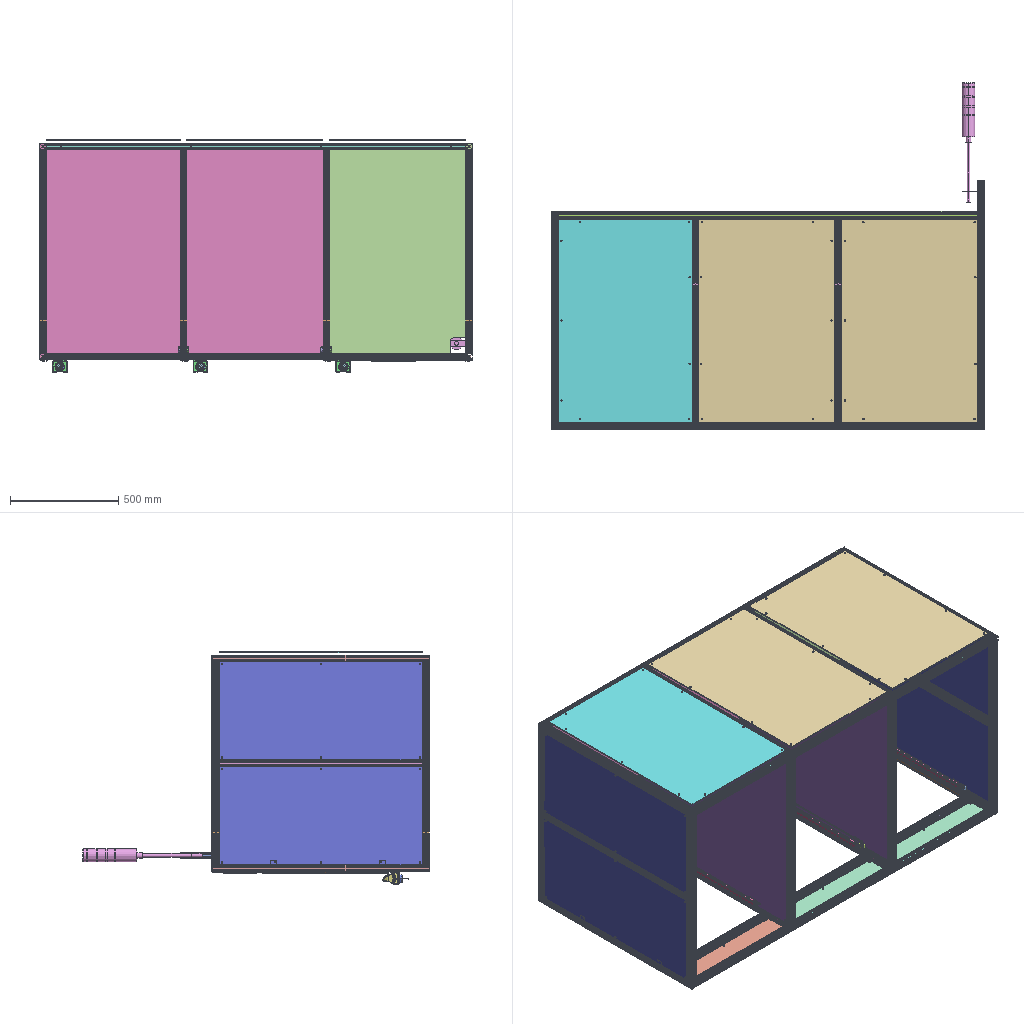Assembly | SolidWorks | 37 different items | 93 placed | box 2000 x 1600 x 1073 mm
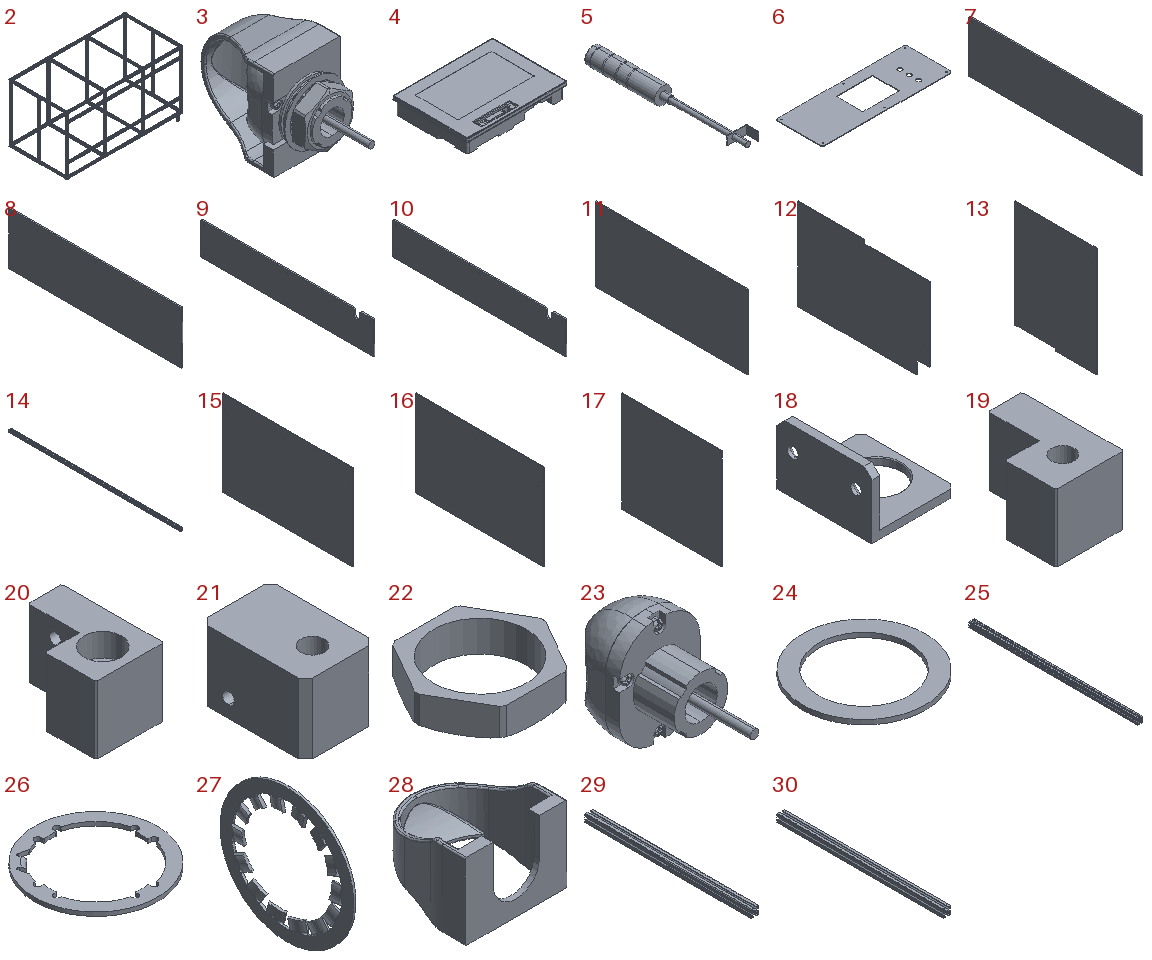Parts list (item | name | quantity | parent item | size | volume | features):
1 | (subassembly) | x2 | - | - | - | features RefAxis 3
2 | (subassembly) | x1 | - | 2000 x 1000 x 1150 mm | 9577291 mm3 | -
3 | (subassembly) | x3 | - | 51 x 119.5 x 68 mm | 99680 mm3 | features RefAxis 3
4 | - | x1 | - | 203 x 152 x 35.35 mm | 852828 mm3 | features BaseBody 1
5 | - | x1 | - | 74 x 551.1 x 60 mm | 791689 mm3 | features Boss 11, ICE 3, BossThin 1, Cut 1, Fillet 1, Shell 1, Sweep 1
6 | - | x1 | - | 690 x 250 x 3 mm | 429850 mm3 | features ICE 2, Extrusion 1, Fillet 1, HoleWzd 1
7 | - | x1 | - | 5 x 628 x 188 mm | 589462 mm3 | features Chamfer 1, Extrusion 1, ICE 1
8 | - | x1 | - | 5 x 618 x 188 mm | 580062 mm3 | features Chamfer 1, Extrusion 1, ICE 1
9 | - | x2 | - | 5 x 628 x 118 mm | 366831 mm3 | features Chamfer 2, ICE 2, Extrusion 1
10 | - | x1 | - | 5 x 628 x 118 mm | 366831 mm3 | features Chamfer 2, ICE 2, Extrusion 1
11 | - | x4 | - | 5 x 937 x 453 mm | 2121447 mm3 | features Chamfer 1, Extrusion 1, ICE 1
12 | - | x1 | - | 5 x 1000 x 690 mm | 3324176 mm3 | features Chamfer 2, Fillet 2, ICE 2, Cut 1, Extrusion 1, HoleWzd 1
13 | - | x1 | - | 5 x 1000 x 1340 mm | 6624000 mm3 | features Chamfer 2, Fillet 2, ICE 2, Extrusion 1
14 | - | x2 | in 2 | 30 x 1940 x 30 mm | 645123 mm3 | features Extrusion 1
15 | - | x1 | - | 5 x 938 x 618 mm | 2897138 mm3 | features Chamfer 1, Extrusion 1, ICE 1
16 | - | x2 | - | 5 x 938 x 628 mm | 2944038 mm3 | features Chamfer 1, Extrusion 1, ICE 1
17 | - | x2 | - | 5 x 937 x 938 mm | 4393672 mm3 | features Chamfer 1, Extrusion 1, ICE 1
18 | - | x3 | - | 53 x 60 x 40 mm | 21818 mm3 | features Chamfer 3, Extrusion 1, HoleWzd 1, ICE 1
19 | - | x2 | - | 20 x 30 x 20 mm | 7804 mm3 | features HoleWzd 2, Chamfer 1, Extrusion 1, ICE 1
20 | - | x2 | - | 20 x 30 x 20 mm | 7804 mm3 | features MirrorStock 1
21 | - | x4 | - | 20 x 30 x 20 mm | 10571 mm3 | features HoleWzd 2, Chamfer 1, Extrusion 1
22 | - | x3 | in 3 | 40.6 x 36 x 10 mm | 4057 mm3 | features RefAxis 3, BaseBody 1
23 | - | x3 | in 3 | 45 x 85.792 x 60 mm | 63985 mm3 | features RefAxis 3, BaseBody 1
24 | - | x3 | in 3 | 42 x 42 x 1.6 mm | 1009 mm3 | features RefAxis 3, BaseBody 1
25 | - | x6 | in 2 | 30 x 940 x 30 mm | 312585 mm3 | features Extrusion 1
26 | - | x3 | in 3 | 38 x 38 x 3.2 mm | 486.379 mm3 | features RefAxis 3, BaseBody 1
27 | - | x3 | in 3 | 2 x 46 x 46 mm | 665.952 mm3 | features RefAxis 3, BaseBody 1
28 | - | x3 | in 3 | 68 x 70 x 51 mm | 29414 mm3 | features RefAxis 3, BaseBody 1
29 | - | x2 | in 2 | 30 x 620 x 30 mm | 206173 mm3 | features Extrusion 1
30 | - | x2 | in 2 | 30 x 630 x 30 mm | 209499 mm3 | features Extrusion 1
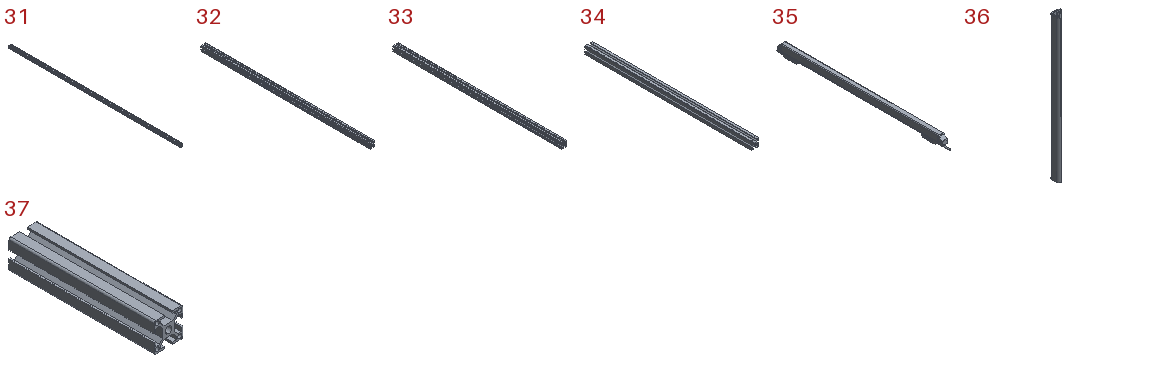31 | - | x2 | in 2 | 30 x 1940 x 30 mm | 644146 mm3 | features Extrusion 1, HoleWzd 1
32 | - | x4 | in 2 | 30 x 1000 x 30 mm | 332538 mm3 | features Extrusion 1
33 | - | x8 | in 2 | 30 x 940 x 30 mm | 311608 mm3 | features Extrusion 1, HoleWzd 1
34 | - | x2 | in 2 | 30 x 630 x 30 mm | 209499 mm3 | features Extrusion 1
35 | - | x6 | - | 15 x 516.175 x 30 mm | 163746 mm3 | features BaseBody 3
36 | - | x4 | - | 37 x 37 x 530 mm | 171468 mm3 | features BaseBody 1, MoveFace 1
37 | - | x1 | in 2 | 30 x 150 x 30 mm | 49881 mm3 | features Extrusion 1
Mates (type | each side: item.copy, entity, surface, feature):
In the top assembly
Coincident | 32.1 face plane Extrude 1 | 6.1 face plane Boss-Extrude 1
Coincident | 14.1 face plane Extrude 1 | 6.1 face plane Boss-Extrude 1
Coincident | 6.1 face plane Boss-Extrude 1 | 4.1 face plane Import 1
Coincident | 6.1 face plane Cut-Extrude 1 | 4.1 face plane Import 1 | 2 times
Coincident | 37.1 face plane Extrude 1 | 5.1 face plane Extrude-Thin Wall 1
Width | 37.1 face plane Extrude 1 | 37.1 face plane Extrude 1 | 5.1 face plane Extrude-Thin Wall 1 | 5.1 face plane Extrude-Thin Wall 1
DistanceDim | 5.1 face plane Extrude 11 | 33.1 face plane Extrude 1
Coincident | 31.1 face plane Extrude 1 | 9.1 face plane Boss-Extrude 1
DistanceDim | 32.1 face plane Extrude 1 | 9.1 face plane Boss-Extrude 1
Coincident | 33.2 face plane Extrude 1 | 11.1 face plane Boss-Extrude 1
DistanceDim | 33.2 face plane Extrude 1 | 11.1 face plane Boss-Extrude 1
DistanceDim | 11.1 face plane Boss-Extrude 1 | 25.1 face plane Extrude 1
Coincident | assembly face | 12.1 face plane Boss-Extrude 1
Coincident | 32.2 face plane Extrude 1 | 12.1 face plane Boss-Extrude 1
Coincident | 33.1 face plane Extrude 1 | 12.1 face plane Boss-Extrude 1
Coincident | 33.3 face plane Extrude 1 | 12.1 face plane Boss-Extrude 1
Coincident | 33.4 face plane Extrude 1 | 13.1 face plane Boss-Extrude 1
Coincident | 14.2 face plane Extrude 1 | 13.1 face plane Boss-Extrude 1
Concentric | 19.1 face cylinder M4 Tapped Hole 1 | 35.1 face cylinder Input 2
Coincident | 19.1 face plane Cut-Extrude 1 | 35.1 face plane Input 2
Concentric | 20.1 face cylinder XXXXXXXXXXXXXXVJTL6_Mirror | 35.1 edge
Coincident | 20.1 face plane XXXXXXXXXXXXXXVJTL6_Mirror | 35.1 face plane Input 1
Parallel | 19.1 face plane Boss-Extrude 1 | 35.1 face plane Input 3
Parallel | 20.1 face plane XXXXXXXXXXXXXXVJTL6_Mirror | 35.1 face plane Input 3
Coincident | 19.2 face plane Cut-Extrude 1 | 35.2 face plane Input 2
Concentric | 20.2 face cylinder XXXXXXXXXXXXXXVJTL6_Mirror | 35.2 edge
Concentric | 19.2 face cylinder M4 Tapped Hole 1 | 35.2 face cylinder Input 2
Parallel | 19.2 face plane Boss-Extrude 1 | 35.2 face plane Input 3
Parallel | 20.2 face plane XXXXXXXXXXXXXXVJTL6_Mirror | 35.2 face plane Input 3
Coincident | 20.2 face plane XXXXXXXXXXXXXXVJTL6_Mirror | 35.2 face plane Input 1
Coincident | 32.1 face plane Extrude 1 | 19.1 face plane Boss-Extrude 1
Coincident | 32.1 face plane Extrude 1 | 35.1 face plane Input 3
Coincident | 25.2 face plane Extrude 1 | 36.1 face plane Input 1 | 2 times
Coincident | 32.1 face plane Extrude 1 | 36.2 face plane Input 1 | 2 times
Coincident | 36.1 face plane Input 1 | 36.2 face plane Input 1
Coincident | 25.3 face plane Extrude 1 | 36.3 face plane Input 1 | 2 times
Coincident | 32.3 face plane Extrude 1 | 36.4 face plane Input 1 | 2 times
DistanceDim | 32.3 face plane Extrude 1 | 20.2 face plane XXXXXXXXXXXXXXVJTL6_Mirror
Coincident | 32.3 face plane Extrude 1 | 20.2 face plane XXXXXXXXXXXXXXVJTL6_Mirror
DistanceDim | 9.1 face plane Boss-Extrude 1 | 31.1 face plane Extrude 1
Concentric | 35.3 face cylinder Input 2 | 21.1 face cylinder M4 Tapped Hole 1
Coincident | 35.3 face plane Input 2 | 21.1 face plane Boss-Extrude 1
Concentric | 35.4 face cylinder Input 1 | 21.1 face cylinder M4 Tapped Hole 1
Coincident | 35.4 face plane Input 1 | 21.1 face plane Boss-Extrude 1
Parallel | 35.3 face plane Input 3 | 21.1 face plane Boss-Extrude 1
Coincident | 35.3 face plane Input 3 | 35.4 face plane Input 3
Concentric | 35.4 face cylinder Input 2 | 21.2 face cylinder M4 Tapped Hole 1
Coincident | 35.4 face plane Input 2 | 21.2 face plane Boss-Extrude 1
Coincident | 21.3 face plane Boss-Extrude 1 | 35.5 face plane Input 1
Concentric | 21.3 face cylinder M4 Tapped Hole 1 | 35.5 face cylinder Input 1
Coincident | 21.3 face plane Boss-Extrude 1 | 35.6 face plane Input 2
Parallel | 21.3 face plane Boss-Extrude 1 | 35.6 face plane Input 3
Concentric | 21.3 face cylinder M4 Tapped Hole 1 | 35.6 face cylinder Input 2
Coincident | 35.5 face plane Input 3 | 35.6 face plane Input 3
Concentric | 21.4 face cylinder M4 Tapped Hole 1 | 35.5 face cylinder Input 2
Coincident | 21.4 face plane Boss-Extrude 1 | 35.5 face plane Input 2
Coincident | 25.2 face plane Extrude 1 | 21.1 face plane Boss-Extrude 1
DistanceDim | 21.1 face plane Boss-Extrude 1 | 25.2 face plane Extrude 1
Coincident | 25.3 face plane Extrude 1 | 21.3 face plane Boss-Extrude 1
DistanceDim | 21.3 face plane Boss-Extrude 1 | 25.3 face plane Extrude 1
Coincident | 19.1 face plane Boss-Extrude 1 | 21.1 face plane Boss-Extrude 1
Coincident | 21.1 face plane Boss-Extrude 1 | 21.3 face plane Boss-Extrude 1
Coincident | 20.2 face plane XXXXXXXXXXXXXXVJTL6_Mirror | 21.3 face plane Boss-Extrude 1
Coincident | 36.1 face plane Input 1 | 21.1 face plane Boss-Extrude 1
Coincident | 6.1 face plane Boss-Extrude 1 | 32.1 face plane Extrude 1
Coincident | 11.2 face plane Boss-Extrude 1 | 11.1 face plane Boss-Extrude 1
DistanceDim | 11.2 face plane Boss-Extrude 1 | 33.1 face plane Extrude 1
DistanceDim | 11.2 face plane Boss-Extrude 1 | 32.2 face plane Extrude 1
Coincident | 32.3 face plane Extrude 1 | 11.3 face plane Boss-Extrude 1
DistanceDim | 11.3 face plane Boss-Extrude 1 | 33.4 face plane Extrude 1
DistanceDim | 11.3 face plane Boss-Extrude 1 | 32.3 face plane Extrude 1
Coincident | 11.3 face plane Boss-Extrude 1 | 11.4 face plane Boss-Extrude 1
DistanceDim | 33.4 face plane Extrude 1 | 11.4 face plane Boss-Extrude 1
DistanceDim | 11.4 face plane Boss-Extrude 1 | 32.4 face plane Extrude 1
Coincident | 25.4 face plane Extrude 1 | 17.1 face plane Boss-Extrude 1
DistanceDim | 33.3 face plane Extrude 1 | 17.1 face plane Boss-Extrude 1
DistanceDim | 25.4 face plane Extrude 1 | 17.1 face plane Boss-Extrude 1
Coincident | 25.5 face plane Extrude 1 | 17.2 face plane Boss-Extrude 1
DistanceDim | 17.2 face plane Boss-Extrude 1 | 33.5 face plane Extrude 1
DistanceDim | 25.3 face plane Extrude 1 | 17.2 face plane Boss-Extrude 1
Coincident | 9.1 face plane Boss-Extrude 1 | 9.2 face plane Boss-Extrude 1
DistanceDim | 9.2 face plane Boss-Extrude 1 | 30.1 face plane Extrude 1
DistanceDim | 9.2 face plane Boss-Extrude 1 | 25.3 face plane Extrude 1
Coincident | 9.2 face plane Boss-Extrude 1 | 10.1 face plane Boss-Extrude 1
DistanceDim | 10.1 face plane Boss-Extrude 1 | 29.1 face plane Extrude 1
DistanceDim | 10.1 face plane Boss-Extrude 1 | 32.3 face plane Extrude 1
Concentric | 18.1 face cylinder Cut-Extrude 1 | 24.1 face cylinder Input 1
Coincident | 18.1 face plane Boss-Extrude 1 | 28.1 face plane Input 1
Parallel | 18.1 face plane Boss-Extrude 1 | 28.1 face plane Input 1
Coincident | 34.1 face plane Extrude 1 | 18.1 face plane Boss-Extrude 1 | 2 times
DistanceDim | 23.1 face cylinder Input 1 | 25.2 face plane Extrude 1
Concentric | 18.2 face cylinder Cut-Extrude 1 | 26.1 face cylinder Input 1
Coincident | 18.2 face plane Boss-Extrude 1 | 28.2 face plane Input 1
Parallel | 18.2 face plane Boss-Extrude 1 | 28.2 face plane Input 1
Concentric | 18.3 face cylinder Cut-Extrude 1 | 26.2 face cylinder Input 1
Coincident | 18.3 face plane Boss-Extrude 1 | 28.3 face plane Input 1
Parallel | 18.3 face plane Boss-Extrude 1 | 28.3 face plane Input 1
Coincident | 30.1 face plane Extrude 1 | 18.2 face plane Boss-Extrude 1 | 2 times
DistanceDim | 23.2 face cylinder Input 1 | 25.3 face plane Extrude 1
Coincident | 29.1 face plane Extrude 1 | 18.3 face plane Boss-Extrude 1 | 2 times
DistanceDim | 23.3 face cylinder Input 1 | 32.3 face plane Extrude 1
DistanceDim | 16.1 face plane Boss-Extrude 1 | 14.2 face plane Extrude 1
DistanceDim | 16.1 face plane Boss-Extrude 1 | 25.5 face plane Extrude 1
Coincident | 16.1 face plane Boss-Extrude 1 | 16.2 face plane Boss-Extrude 1
DistanceDim | 16.2 face plane Boss-Extrude 1 | 14.2 face plane Extrude 1
DistanceDim | 16.2 face plane Boss-Extrude 1 | 32.2 face plane Extrude 1
Coincident | 14.1 face plane Extrude 1 | 7.1 face plane Boss-Extrude 1
DistanceDim | 7.1 face plane Boss-Extrude 1 | 30.2 face plane Extrude 1
DistanceDim | 7.1 face plane Boss-Extrude 1 | 25.3 face plane Extrude 1
Coincident | 7.1 face plane Boss-Extrude 1 | 8.1 face plane Boss-Extrude 1
DistanceDim | 8.1 face plane Boss-Extrude 1 | 14.1 face plane Extrude 1
DistanceDim | 8.1 face plane Boss-Extrude 1 | 32.3 face plane Extrude 1
Coincident | assembly face | 4.1 face plane Import 1 | 3 times
Coincident | 16.1 face plane Boss-Extrude 1 | 15.1 face plane Boss-Extrude 1
DistanceDim | 15.1 face plane Boss-Extrude 1 | 14.2 face plane Extrude 1
DistanceDim | 15.1 face plane Boss-Extrude 1 | 32.4 face plane Extrude 1
In subassembly 2
Coincident | 31.2 face plane Extrude 1 | 25.6 face plane Extrude 1 | 2 times
Coincident | 32.5 face plane Extrude 1 | 33.6 face plane Extrude 1 | 3 times
Coincident | 14.3 face plane Extrude 1 | 32.6 face plane Extrude 1 | 3 times
DistanceDim | 31.3 face plane Extrude 1 | 14.3 face plane Extrude 1
Coincident | 14.4 face plane Extrude 1 | 32.5 face plane Extrude 1 | 3 times
Coincident | 31.2 face plane Extrude 1 | 25.7 face plane Extrude 1 | 2 times
Coincident | 14.4 face plane Extrude 1 | 33.7 face plane Extrude 1 | 2 times
Coincident | 31.2 face plane Extrude 1 | 32.5 face plane Extrude 1
Coincident | 31.2 face plane Extrude 1 | 31.3 face plane Extrude 1
Coincident | 32.6 face plane Extrude 1 | 33.8 face plane Extrude 1 | 3 times
Coincident | 33.8 face plane Extrude 1 | 25.8 face plane Extrude 1 | 2 times
Width | 32.5 face plane Extrude 1 | 32.6 face plane Extrude 1 | 25.8 face plane Extrude 1 | 25.8 face plane Extrude 1
Coincident | 32.6 face plane Extrude 1 | 34.2 face plane Extrude 1 | 2 times
Coincident | 31.3 face plane Extrude 1 | 25.9 face plane Extrude 1 | 2 times
Coincident | 14.4 face plane Extrude 1 | 33.9 face plane Extrude 1 | 2 times
Coincident | 31.3 face plane Extrude 1 | 32.7 face plane Extrude 1 | 3 times
Coincident | 31.2 face plane Extrude 1 | 32.8 face plane Extrude 1 | 3 times
Coincident | 14.4 face plane Extrude 1 | 32.8 face plane Extrude 1
Coincident | 32.6 face plane Extrude 1 | 33.6 face plane Extrude 1 | 2 times
Coincident | 31.3 face plane Extrude 1 | 32.6 face plane Extrude 1 | 2 times
Coincident | 33.7 face plane Extrude 1 | 32.8 face plane Extrude 1
Coincident | 33.7 face plane Extrude 1 | 32.7 face plane Extrude 1
Coincident | 25.6 face plane Extrude 1 | 25.9 face plane Extrude 1
Coincident | 25.9 face plane Extrude 1 | 33.9 face plane Extrude 1
Coincident | 33.6 face plane Extrude 1 | 33.10 face plane Extrude 1
Coincident | 14.3 face plane Extrude 1 | 33.10 face plane Extrude 1
DistanceDim | 37.2 face plane Extrude 1 | 32.6 face plane Extrude 1
Coincident | 33.6 face plane Extrude 1 | 37.2 face plane Extrude 1 | 2 times
Coincident | 25.10 face plane Extrude 1 | 34.3 face plane Extrude 1 | 2 times
Coincident | 31.3 face plane Extrude 1 | 34.3 face plane Extrude 1
Coincident | 32.6 face plane Extrude 1 | 34.3 face plane Extrude 1
Coincident | 34.3 face plane Extrude 1 | 30.3 face plane Extrude 1 | 2 times
Coincident | 33.11 face plane Extrude 1 | 33.12 face plane Extrude 1
Coincident | 33.13 face plane Extrude 1 | 33.12 face plane Extrude 1
Coincident | 33.12 face plane Extrude 1 | 33.11 face plane Extrude 1
Coincident | 33.12 face plane Extrude 1 | 33.13 face plane Extrude 1
Coincident | 25.7 face plane Extrude 1 | 33.12 face plane Extrude 1
Coincident | 25.6 face plane Extrude 1 | 33.13 face plane Extrude 1 | 2 times
Coincident | 31.2 face plane Extrude 1 | 33.11 face plane Extrude 1
Coincident | 32.8 face plane Extrude 1 | 33.11 face plane Extrude 1 | 2 times
Coincident | 25.10 face plane Extrude 1 | 33.12 face plane Extrude 1
Coincident | 25.7 face plane Extrude 1 | 33.10 face plane Extrude 1
Coincident | 25.10 face plane Extrude 1 | 31.3 face plane Extrude 1
Coincident | 14.3 face plane Extrude 1 | 25.10 face plane Extrude 1
Coincident | 25.10 face plane Extrude 1 | 30.3 face plane Extrude 1
Coincident | 25.9 face plane Extrude 1 | 30.3 face plane Extrude 1
Coincident | 25.9 face plane Extrude 1 | 29.2 face plane Extrude 1
Coincident | 34.2 face plane Extrude 1 | 30.4 face plane Extrude 1 | 2 times
Coincident | 25.10 face plane Extrude 1 | 30.4 face plane Extrude 1
Coincident | 30.4 face plane Extrude 1 | 29.3 face plane Extrude 1 | 2 times
Coincident | 25.9 face plane Extrude 1 | 29.3 face plane Extrude 1
DistanceDim | 34.2 face plane Extrude 1 | 14.3 face plane Extrude 1
DistanceDim | 34.3 face plane Extrude 1 | 31.3 face plane Extrude 1
Coincident | 32.7 face plane Extrude 1 | 25.11 face plane Extrude 1
Coincident | 33.11 face plane Extrude 1 | 25.11 face plane Extrude 1
Coincident | 25.8 face plane Extrude 1 | 25.11 face plane Extrude 1